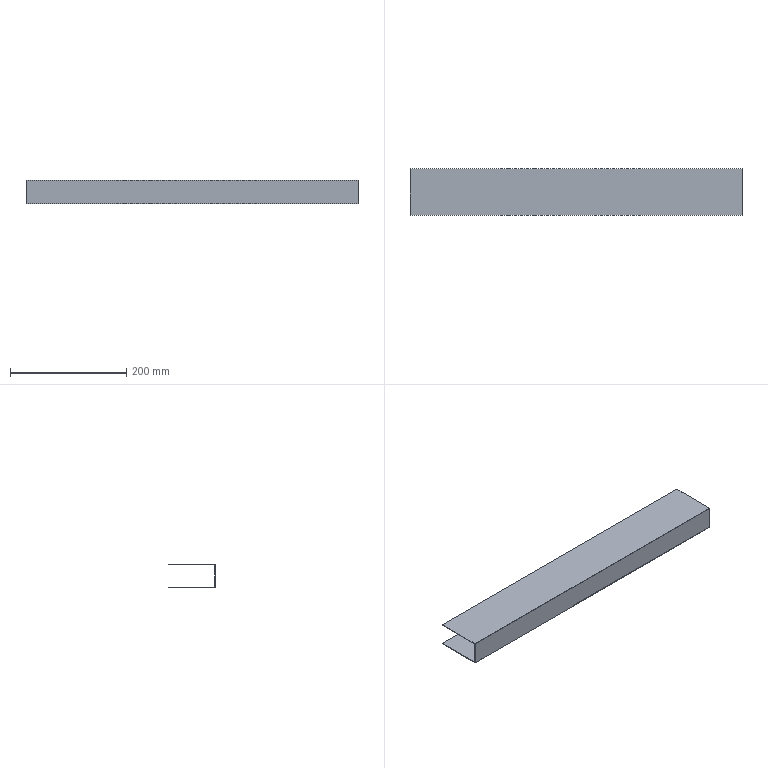Part | SolidWorks | features BaseBody 1 | 1 solid | 10 faces | box 570 x 80 x 40 mm | volume 112860 mm3 | plane 10
STEP:
#1=CARTESIAN_POINT('',(0.,1.,19.));
#2=VERTEX_POINT('',#1);
#3=CARTESIAN_POINT('',(0.,80.,19.));
#4=VERTEX_POINT('',#3);
#5=CARTESIAN_POINT('',(0.,0.,19.));
#6=DIRECTION('',(0.,1.,0.));
#7=VECTOR('',#6,1000.);
#8=LINE('',#5,#7);
#9=EDGE_CURVE('',#2,#4,#8,.T.);
#10=ORIENTED_EDGE('',*,*,#9,.F.);
#11=CARTESIAN_POINT('',(0.,1.,-19.));
#12=VERTEX_POINT('',#11);
#13=CARTESIAN_POINT('',(0.,1.,20.));
#14=DIRECTION('',(0.,0.,1.));
#15=VECTOR('',#14,1000.);
#16=LINE('',#13,#15);
#17=EDGE_CURVE('',#12,#2,#16,.T.);
#18=ORIENTED_EDGE('',*,*,#17,.F.);
#19=CARTESIAN_POINT('',(0.,80.,-19.));
#20=VERTEX_POINT('',#19);
#21=CARTESIAN_POINT('',(0.,0.,-19.));
#22=DIRECTION('',(0.,-1.,0.));
#23=VECTOR('',#22,1000.);
#24=LINE('',#21,#23);
#25=EDGE_CURVE('',#20,#12,#24,.T.);
#26=ORIENTED_EDGE('',*,*,#25,.F.);
#27=CARTESIAN_POINT('',(0.,80.,-20.));
#28=VERTEX_POINT('',#27);
#29=CARTESIAN_POINT('',(0.,80.,-19.));
#30=DIRECTION('',(0.,0.,-1.));
#31=VECTOR('',#30,1000.);
#32=LINE('',#29,#31);
#33=EDGE_CURVE('',#20,#28,#32,.T.);
#34=ORIENTED_EDGE('',*,*,#33,.T.);
#35=CARTESIAN_POINT('',(0.,0.,-20.));
#36=VERTEX_POINT('',#35);
#37=CARTESIAN_POINT('',(0.,0.,-20.));
#38=DIRECTION('',(0.,-1.,0.));
#39=VECTOR('',#38,1000.);
#40=LINE('',#37,#39);
#41=EDGE_CURVE('',#28,#36,#40,.T.);
#42=ORIENTED_EDGE('',*,*,#41,.T.);
#43=CARTESIAN_POINT('',(0.,0.,20.));
#44=VERTEX_POINT('',#43);
#45=CARTESIAN_POINT('',(0.,0.,20.));
#46=DIRECTION('',(0.,0.,1.));
#47=VECTOR('',#46,1000.);
#48=LINE('',#45,#47);
#49=EDGE_CURVE('',#36,#44,#48,.T.);
#50=ORIENTED_EDGE('',*,*,#49,.T.);
#51=CARTESIAN_POINT('',(0.,80.,20.));
#52=VERTEX_POINT('',#51);
#53=CARTESIAN_POINT('',(0.,0.,20.));
#54=DIRECTION('',(0.,1.,0.));
#55=VECTOR('',#54,1000.);
#56=LINE('',#53,#55);
#57=EDGE_CURVE('',#44,#52,#56,.T.);
#58=ORIENTED_EDGE('',*,*,#57,.T.);
#59=CARTESIAN_POINT('',(0.,80.,20.));
#60=DIRECTION('',(0.,0.,-1.));
#61=VECTOR('',#60,1000.);
#62=LINE('',#59,#61);
#63=EDGE_CURVE('',#52,#4,#62,.T.);
#64=ORIENTED_EDGE('',*,*,#63,.T.);
#65=EDGE_LOOP('',(#10,#18,#26,#34,#42,#50,#58,#64));
#66=FACE_OUTER_BOUND('',#65,.T.);
#67=CARTESIAN_POINT('',(0.,0.,0.));
#68=DIRECTION('',(-1.,0.,0.));
#69=DIRECTION('',(0.,0.,1.));
#70=AXIS2_PLACEMENT_3D('',#67,#68,#69);
#71=PLANE('',#70);
#72=ADVANCED_FACE('',(#66),#71,.T.);
#73=CARTESIAN_POINT('',(570.,1.,19.));
#74=VERTEX_POINT('',#73);
#75=CARTESIAN_POINT('',(570.,80.,19.));
#76=VERTEX_POINT('',#75);
#77=CARTESIAN_POINT('',(570.,0.,19.));
#78=DIRECTION('',(0.,1.,0.));
#79=VECTOR('',#78,1000.);
#80=LINE('',#77,#79);
#81=EDGE_CURVE('',#74,#76,#80,.T.);
#82=ORIENTED_EDGE('',*,*,#81,.T.);
#83=CARTESIAN_POINT('',(570.,80.,20.));
#84=VERTEX_POINT('',#83);
#85=CARTESIAN_POINT('',(570.,80.,20.));
#86=DIRECTION('',(0.,0.,-1.));
#87=VECTOR('',#86,1000.);
#88=LINE('',#85,#87);
#89=EDGE_CURVE('',#84,#76,#88,.T.);
#90=ORIENTED_EDGE('',*,*,#89,.F.);
#91=CARTESIAN_POINT('',(570.,0.,20.));
#92=VERTEX_POINT('',#91);
#93=CARTESIAN_POINT('',(570.,0.,20.));
#94=DIRECTION('',(0.,1.,0.));
#95=VECTOR('',#94,1000.);
#96=LINE('',#93,#95);
#97=EDGE_CURVE('',#92,#84,#96,.T.);
#98=ORIENTED_EDGE('',*,*,#97,.F.);
#99=CARTESIAN_POINT('',(570.,0.,-20.));
#100=VERTEX_POINT('',#99);
#101=CARTESIAN_POINT('',(570.,0.,20.));
#102=DIRECTION('',(0.,0.,1.));
#103=VECTOR('',#102,1000.);
#104=LINE('',#101,#103);
#105=EDGE_CURVE('',#100,#92,#104,.T.);
#106=ORIENTED_EDGE('',*,*,#105,.F.);
#107=CARTESIAN_POINT('',(570.,80.,-20.));
#108=VERTEX_POINT('',#107);
#109=CARTESIAN_POINT('',(570.,0.,-20.));
#110=DIRECTION('',(0.,-1.,0.));
#111=VECTOR('',#110,1000.);
#112=LINE('',#109,#111);
#113=EDGE_CURVE('',#108,#100,#112,.T.);
#114=ORIENTED_EDGE('',*,*,#113,.F.);
#115=CARTESIAN_POINT('',(570.,80.,-19.));
#116=VERTEX_POINT('',#115);
#117=CARTESIAN_POINT('',(570.,80.,-19.));
#118=DIRECTION('',(0.,0.,-1.));
#119=VECTOR('',#118,1000.);
#120=LINE('',#117,#119);
#121=EDGE_CURVE('',#116,#108,#120,.T.);
#122=ORIENTED_EDGE('',*,*,#121,.F.);
#123=CARTESIAN_POINT('',(570.,1.,-19.));
#124=VERTEX_POINT('',#123);
#125=CARTESIAN_POINT('',(570.,0.,-19.));
#126=DIRECTION('',(0.,-1.,0.));
#127=VECTOR('',#126,1000.);
#128=LINE('',#125,#127);
#129=EDGE_CURVE('',#116,#124,#128,.T.);
#130=ORIENTED_EDGE('',*,*,#129,.T.);
#131=CARTESIAN_POINT('',(570.,1.,20.));
#132=DIRECTION('',(0.,0.,1.));
#133=VECTOR('',#132,1000.);
#134=LINE('',#131,#133);
#135=EDGE_CURVE('',#124,#74,#134,.T.);
#136=ORIENTED_EDGE('',*,*,#135,.T.);
#137=EDGE_LOOP('',(#82,#90,#98,#106,#114,#122,#130,#136));
#138=FACE_OUTER_BOUND('',#137,.T.);
#139=CARTESIAN_POINT('',(570.,0.,0.));
#140=DIRECTION('',(-1.,0.,0.));
#141=DIRECTION('',(0.,0.,1.));
#142=AXIS2_PLACEMENT_3D('',#139,#140,#141);
#143=PLANE('',#142);
#144=ADVANCED_FACE('',(#138),#143,.F.);
#145=ORIENTED_EDGE('',*,*,#17,.T.);
#146=CARTESIAN_POINT('',(570.,1.,19.));
#147=DIRECTION('',(-1.,0.,0.));
#148=VECTOR('',#147,1000.);
#149=LINE('',#146,#148);
#150=EDGE_CURVE('',#74,#2,#149,.T.);
#151=ORIENTED_EDGE('',*,*,#150,.F.);
#152=ORIENTED_EDGE('',*,*,#135,.F.);
#153=CARTESIAN_POINT('',(570.,1.,-19.));
#154=DIRECTION('',(-1.,0.,0.));
#155=VECTOR('',#154,1000.);
#156=LINE('',#153,#155);
#157=EDGE_CURVE('',#124,#12,#156,.T.);
#158=ORIENTED_EDGE('',*,*,#157,.T.);
#159=EDGE_LOOP('',(#145,#151,#152,#158));
#160=FACE_OUTER_BOUND('',#159,.T.);
#161=CARTESIAN_POINT('',(570.,1.,20.));
#162=DIRECTION('',(0.,-1.,0.));
#163=DIRECTION('',(0.,0.,-1.));
#164=AXIS2_PLACEMENT_3D('',#161,#162,#163);
#165=PLANE('',#164);
#166=ADVANCED_FACE('',(#160),#165,.F.);
#167=ORIENTED_EDGE('',*,*,#25,.T.);
#168=ORIENTED_EDGE('',*,*,#157,.F.);
#169=ORIENTED_EDGE('',*,*,#129,.F.);
#170=CARTESIAN_POINT('',(570.,80.,-19.));
#171=DIRECTION('',(-1.,0.,0.));
#172=VECTOR('',#171,1000.);
#173=LINE('',#170,#172);
#174=EDGE_CURVE('',#116,#20,#173,.T.);
#175=ORIENTED_EDGE('',*,*,#174,.T.);
#176=EDGE_LOOP('',(#167,#168,#169,#175));
#177=FACE_OUTER_BOUND('',#176,.T.);
#178=CARTESIAN_POINT('',(570.,0.,-19.));
#179=DIRECTION('',(0.,0.,-1.));
#180=DIRECTION('',(0.,-1.,0.));
#181=AXIS2_PLACEMENT_3D('',#178,#179,#180);
#182=PLANE('',#181);
#183=ADVANCED_FACE('',(#177),#182,.F.);
#184=ORIENTED_EDGE('',*,*,#33,.F.);
#185=ORIENTED_EDGE('',*,*,#174,.F.);
#186=ORIENTED_EDGE('',*,*,#121,.T.);
#187=CARTESIAN_POINT('',(570.,80.,-20.));
#188=DIRECTION('',(-1.,0.,0.));
#189=VECTOR('',#188,1000.);
#190=LINE('',#187,#189);
#191=EDGE_CURVE('',#108,#28,#190,.T.);
#192=ORIENTED_EDGE('',*,*,#191,.T.);
#193=EDGE_LOOP('',(#184,#185,#186,#192));
#194=FACE_OUTER_BOUND('',#193,.T.);
#195=CARTESIAN_POINT('',(570.,80.,-19.));
#196=DIRECTION('',(0.,1.,0.));
#197=DIRECTION('',(1.,0.,0.));
#198=AXIS2_PLACEMENT_3D('',#195,#196,#197);
#199=PLANE('',#198);
#200=ADVANCED_FACE('',(#194),#199,.T.);
#201=ORIENTED_EDGE('',*,*,#41,.F.);
#202=ORIENTED_EDGE('',*,*,#191,.F.);
#203=ORIENTED_EDGE('',*,*,#113,.T.);
#204=CARTESIAN_POINT('',(570.,0.,-20.));
#205=DIRECTION('',(-1.,0.,0.));
#206=VECTOR('',#205,1000.);
#207=LINE('',#204,#206);
#208=EDGE_CURVE('',#100,#36,#207,.T.);
#209=ORIENTED_EDGE('',*,*,#208,.T.);
#210=EDGE_LOOP('',(#201,#202,#203,#209));
#211=FACE_OUTER_BOUND('',#210,.T.);
#212=CARTESIAN_POINT('',(570.,0.,-20.));
#213=DIRECTION('',(0.,0.,-1.));
#214=DIRECTION('',(0.,-1.,0.));
#215=AXIS2_PLACEMENT_3D('',#212,#213,#214);
#216=PLANE('',#215);
#217=ADVANCED_FACE('',(#211),#216,.T.);
#218=ORIENTED_EDGE('',*,*,#49,.F.);
#219=ORIENTED_EDGE('',*,*,#208,.F.);
#220=ORIENTED_EDGE('',*,*,#105,.T.);
#221=CARTESIAN_POINT('',(570.,0.,20.));
#222=DIRECTION('',(-1.,0.,0.));
#223=VECTOR('',#222,1000.);
#224=LINE('',#221,#223);
#225=EDGE_CURVE('',#92,#44,#224,.T.);
#226=ORIENTED_EDGE('',*,*,#225,.T.);
#227=EDGE_LOOP('',(#218,#219,#220,#226));
#228=FACE_OUTER_BOUND('',#227,.T.);
#229=CARTESIAN_POINT('',(570.,0.,20.));
#230=DIRECTION('',(0.,-1.,0.));
#231=DIRECTION('',(0.,0.,-1.));
#232=AXIS2_PLACEMENT_3D('',#229,#230,#231);
#233=PLANE('',#232);
#234=ADVANCED_FACE('',(#228),#233,.T.);
#235=ORIENTED_EDGE('',*,*,#57,.F.);
#236=ORIENTED_EDGE('',*,*,#225,.F.);
#237=ORIENTED_EDGE('',*,*,#97,.T.);
#238=CARTESIAN_POINT('',(570.,80.,20.));
#239=DIRECTION('',(-1.,0.,0.));
#240=VECTOR('',#239,1000.);
#241=LINE('',#238,#240);
#242=EDGE_CURVE('',#84,#52,#241,.T.);
#243=ORIENTED_EDGE('',*,*,#242,.T.);
#244=EDGE_LOOP('',(#235,#236,#237,#243));
#245=FACE_OUTER_BOUND('',#244,.T.);
#246=CARTESIAN_POINT('',(570.,0.,20.));
#247=DIRECTION('',(0.,0.,1.));
#248=DIRECTION('',(0.,-1.,0.));
#249=AXIS2_PLACEMENT_3D('',#246,#247,#248);
#250=PLANE('',#249);
#251=ADVANCED_FACE('',(#245),#250,.T.);
#252=ORIENTED_EDGE('',*,*,#63,.F.);
#253=ORIENTED_EDGE('',*,*,#242,.F.);
#254=ORIENTED_EDGE('',*,*,#89,.T.);
#255=CARTESIAN_POINT('',(570.,80.,19.));
#256=DIRECTION('',(-1.,0.,0.));
#257=VECTOR('',#256,1000.);
#258=LINE('',#255,#257);
#259=EDGE_CURVE('',#76,#4,#258,.T.);
#260=ORIENTED_EDGE('',*,*,#259,.T.);
#261=EDGE_LOOP('',(#252,#253,#254,#260));
#262=FACE_OUTER_BOUND('',#261,.T.);
#263=CARTESIAN_POINT('',(570.,80.,20.));
#264=DIRECTION('',(0.,1.,0.));
#265=DIRECTION('',(1.,0.,0.));
#266=AXIS2_PLACEMENT_3D('',#263,#264,#265);
#267=PLANE('',#266);
#268=ADVANCED_FACE('',(#262),#267,.T.);
#269=ORIENTED_EDGE('',*,*,#9,.T.);
#270=ORIENTED_EDGE('',*,*,#259,.F.);
#271=ORIENTED_EDGE('',*,*,#81,.F.);
#272=ORIENTED_EDGE('',*,*,#150,.T.);
#273=EDGE_LOOP('',(#269,#270,#271,#272));
#274=FACE_OUTER_BOUND('',#273,.T.);
#275=CARTESIAN_POINT('',(570.,0.,19.));
#276=DIRECTION('',(0.,0.,1.));
#277=DIRECTION('',(0.,-1.,0.));
#278=AXIS2_PLACEMENT_3D('',#275,#276,#277);
#279=PLANE('',#278);
#280=ADVANCED_FACE('',(#274),#279,.F.);
#281=CLOSED_SHELL('',(#72,#144,#166,#183,#200,#217,#234,#251,#268,#280));
#282=MANIFOLD_SOLID_BREP('',#281);
#283=CARTESIAN_POINT('',(0.,0.,0.));
#284=DIRECTION('',(0.,0.,1.));
#285=DIRECTION('',(1.,0.,0.));
#286=AXIS2_PLACEMENT_3D('',#283,#284,#285);
#287=(LENGTH_UNIT()NAMED_UNIT(*)SI_UNIT(.MILLI.,.METRE.));
#288=UNCERTAINTY_MEASURE_WITH_UNIT(LENGTH_MEASURE(0.00001),#287,'','');
#289=(NAMED_UNIT(*)PLANE_ANGLE_UNIT()SI_UNIT($,.RADIAN.));
#290=(NAMED_UNIT(*)SI_UNIT($,.STERADIAN.)SOLID_ANGLE_UNIT());
#291=(GEOMETRIC_REPRESENTATION_CONTEXT(3)GLOBAL_UNCERTAINTY_ASSIGNED_CONTEXT((#288))GLOBAL_UNIT_ASSIGNED_CONTEXT((#287,#289,#290))REPRESENTATION_CONTEXT('',''));
#292=ADVANCED_BREP_SHAPE_REPRESENTATION('',(#282,#286),#291);